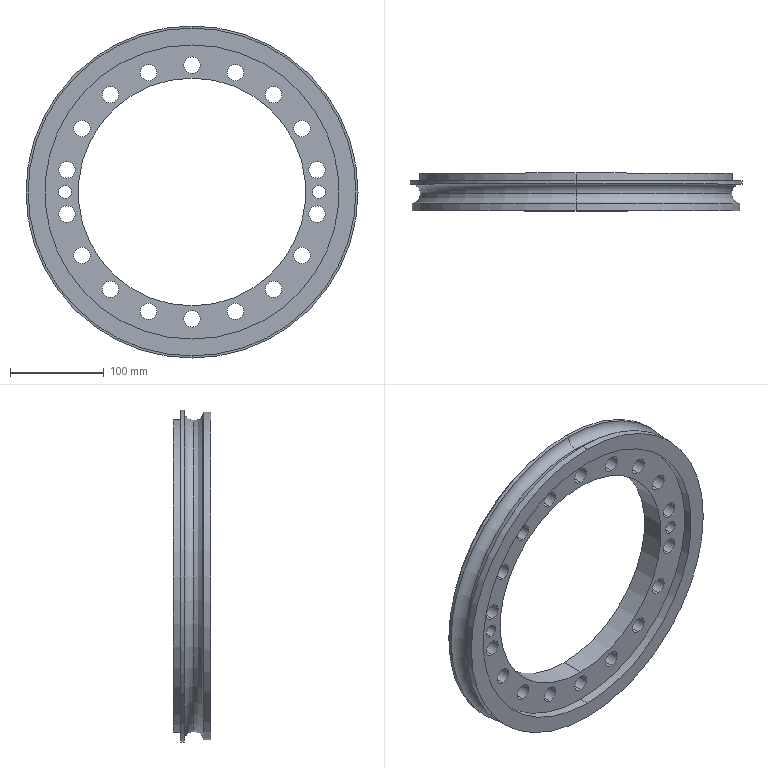Part | SolidWorks | features HoleWzd 3, CirPattern 2, RefAxis 1, Revolution 1 | 1 solid | 109 faces | box 354.4 x 40 x 354.4 mm | volume 1222864 mm3 | cylinder 76 | cone 24 | plane 5 | torus 4 | commonest cylinder face diameters 17.5 x36 9 x24 14 x4 243 x2 298 x2 314 x2